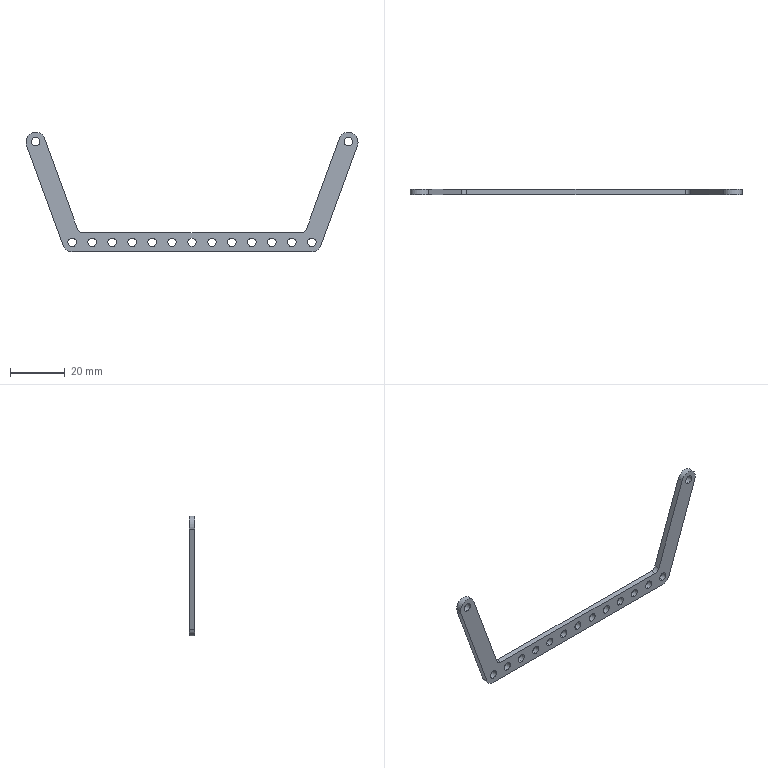Part | SolidWorks | features Extrusion 1, Fillet 1 | 1 solid | 44 faces | box 121 x 2 x 43.639 mm | volume 2162 mm3 | cylinder 36 | plane 8 | commonest cylinder face diameters 3.1 x30 7 x4 4 x2
STEP:
#1=CARTESIAN_POINT('',(57.,2.,-1.55));
#2=VERTEX_POINT('',#1);
#3=CARTESIAN_POINT('',(57.,2.,1.55));
#4=VERTEX_POINT('',#3);
#5=CARTESIAN_POINT('',(57.,2.,0.));
#6=DIRECTION('',(0.,1.,0.));
#7=DIRECTION('',(0.,0.,1.));
#8=AXIS2_PLACEMENT_3D('',#5,#6,#7);
#9=CIRCLE('',#8,1.55);
#10=EDGE_CURVE('',#2,#4,#9,.T.);
#11=ORIENTED_EDGE('',*,*,#10,.T.);
#12=CARTESIAN_POINT('',(57.,0.,1.55));
#13=VERTEX_POINT('',#12);
#14=CARTESIAN_POINT('',(57.,2.,1.55));
#15=DIRECTION('',(0.,-1.,0.));
#16=VECTOR('',#15,1000.);
#17=LINE('',#14,#16);
#18=EDGE_CURVE('',#4,#13,#17,.T.);
#19=ORIENTED_EDGE('',*,*,#18,.T.);
#20=CARTESIAN_POINT('',(57.,0.,-1.55));
#21=VERTEX_POINT('',#20);
#22=CARTESIAN_POINT('',(57.,0.,0.));
#23=DIRECTION('',(0.,1.,0.));
#24=DIRECTION('',(0.,0.,1.));
#25=AXIS2_PLACEMENT_3D('',#22,#23,#24);
#26=CIRCLE('',#25,1.55);
#27=EDGE_CURVE('',#21,#13,#26,.T.);
#28=ORIENTED_EDGE('',*,*,#27,.F.);
#29=CARTESIAN_POINT('',(57.,2.,-1.55));
#30=DIRECTION('',(0.,-1.,0.));
#31=VECTOR('',#30,1000.);
#32=LINE('',#29,#31);
#33=EDGE_CURVE('',#2,#21,#32,.T.);
#34=ORIENTED_EDGE('',*,*,#33,.F.);
#35=EDGE_LOOP('',(#11,#19,#28,#34));
#36=FACE_OUTER_BOUND('',#35,.T.);
#37=CARTESIAN_POINT('',(57.,2.,0.));
#38=DIRECTION('',(0.,-1.,0.));
#39=DIRECTION('',(0.,0.,-1.));
#40=AXIS2_PLACEMENT_3D('',#37,#38,#39);
#41=CYLINDRICAL_SURFACE('',#40,1.55);
#42=ADVANCED_FACE('',(#36),#41,.F.);
#43=CARTESIAN_POINT('',(-57.,2.,1.55));
#44=VERTEX_POINT('',#43);
#45=CARTESIAN_POINT('',(-57.,2.,-1.55));
#46=VERTEX_POINT('',#45);
#47=CARTESIAN_POINT('',(-57.,2.,0.));
#48=DIRECTION('',(0.,-1.,0.));
#49=DIRECTION('',(0.,0.,1.));
#50=AXIS2_PLACEMENT_3D('',#47,#48,#49);
#51=CIRCLE('',#50,1.55);
#52=EDGE_CURVE('',#44,#46,#51,.T.);
#53=ORIENTED_EDGE('',*,*,#52,.F.);
#54=CARTESIAN_POINT('',(-57.,0.,1.55));
#55=VERTEX_POINT('',#54);
#56=CARTESIAN_POINT('',(-57.,2.,1.55));
#57=DIRECTION('',(0.,-1.,0.));
#58=VECTOR('',#57,1000.);
#59=LINE('',#56,#58);
#60=EDGE_CURVE('',#44,#55,#59,.T.);
#61=ORIENTED_EDGE('',*,*,#60,.T.);
#62=CARTESIAN_POINT('',(-57.,0.,-1.55));
#63=VERTEX_POINT('',#62);
#64=CARTESIAN_POINT('',(-57.,0.,0.));
#65=DIRECTION('',(0.,-1.,0.));
#66=DIRECTION('',(0.,0.,1.));
#67=AXIS2_PLACEMENT_3D('',#64,#65,#66);
#68=CIRCLE('',#67,1.55);
#69=EDGE_CURVE('',#55,#63,#68,.T.);
#70=ORIENTED_EDGE('',*,*,#69,.T.);
#71=CARTESIAN_POINT('',(-57.,2.,-1.55));
#72=DIRECTION('',(0.,-1.,0.));
#73=VECTOR('',#72,1000.);
#74=LINE('',#71,#73);
#75=EDGE_CURVE('',#46,#63,#74,.T.);
#76=ORIENTED_EDGE('',*,*,#75,.F.);
#77=EDGE_LOOP('',(#53,#61,#70,#76));
#78=FACE_OUTER_BOUND('',#77,.T.);
#79=CARTESIAN_POINT('',(-57.,2.,0.));
#80=DIRECTION('',(0.,-1.,0.));
#81=DIRECTION('',(0.,0.,-1.));
#82=AXIS2_PLACEMENT_3D('',#79,#80,#81);
#83=CYLINDRICAL_SURFACE('',#82,1.55);
#84=ADVANCED_FACE('',(#78),#83,.F.);
#85=CARTESIAN_POINT('',(-43.665,2.,-35.089));
#86=VERTEX_POINT('',#85);
#87=CARTESIAN_POINT('',(-43.665,2.,-38.189));
#88=VERTEX_POINT('',#87);
#89=CARTESIAN_POINT('',(-43.665,2.,-36.639));
#90=DIRECTION('',(0.,-1.,0.));
#91=DIRECTION('',(0.,0.,1.));
#92=AXIS2_PLACEMENT_3D('',#89,#90,#91);
#93=CIRCLE('',#92,1.55);
#94=EDGE_CURVE('',#86,#88,#93,.T.);
#95=ORIENTED_EDGE('',*,*,#94,.F.);
#96=CARTESIAN_POINT('',(-43.665,0.,-35.089));
#97=VERTEX_POINT('',#96);
#98=CARTESIAN_POINT('',(-43.665,2.,-35.089));
#99=DIRECTION('',(0.,-1.,0.));
#100=VECTOR('',#99,1000.);
#101=LINE('',#98,#100);
#102=EDGE_CURVE('',#86,#97,#101,.T.);
#103=ORIENTED_EDGE('',*,*,#102,.T.);
#104=CARTESIAN_POINT('',(-43.665,0.,-38.189));
#105=VERTEX_POINT('',#104);
#106=CARTESIAN_POINT('',(-43.665,0.,-36.639));
#107=DIRECTION('',(0.,-1.,0.));
#108=DIRECTION('',(0.,0.,1.));
#109=AXIS2_PLACEMENT_3D('',#106,#107,#108);
#110=CIRCLE('',#109,1.55);
#111=EDGE_CURVE('',#97,#105,#110,.T.);
#112=ORIENTED_EDGE('',*,*,#111,.T.);
#113=CARTESIAN_POINT('',(-43.665,2.,-38.189));
#114=DIRECTION('',(0.,-1.,0.));
#115=VECTOR('',#114,1000.);
#116=LINE('',#113,#115);
#117=EDGE_CURVE('',#88,#105,#116,.T.);
#118=ORIENTED_EDGE('',*,*,#117,.F.);
#119=EDGE_LOOP('',(#95,#103,#112,#118));
#120=FACE_OUTER_BOUND('',#119,.T.);
#121=CARTESIAN_POINT('',(-43.665,2.,-36.639));
#122=DIRECTION('',(0.,-1.,0.));
#123=DIRECTION('',(0.,0.,-1.));
#124=AXIS2_PLACEMENT_3D('',#121,#122,#123);
#125=CYLINDRICAL_SURFACE('',#124,1.55);
#126=ADVANCED_FACE('',(#120),#125,.F.);
#127=CARTESIAN_POINT('',(36.388,2.,-38.189));
#128=VERTEX_POINT('',#127);
#129=CARTESIAN_POINT('',(36.388,2.,-35.089));
#130=VERTEX_POINT('',#129);
#131=CARTESIAN_POINT('',(36.388,2.,-36.639));
#132=DIRECTION('',(0.,1.,0.));
#133=DIRECTION('',(0.,0.,1.));
#134=AXIS2_PLACEMENT_3D('',#131,#132,#133);
#135=CIRCLE('',#134,1.55);
#136=EDGE_CURVE('',#128,#130,#135,.T.);
#137=ORIENTED_EDGE('',*,*,#136,.T.);
#138=CARTESIAN_POINT('',(36.388,0.,-35.089));
#139=VERTEX_POINT('',#138);
#140=CARTESIAN_POINT('',(36.388,2.,-35.089));
#141=DIRECTION('',(0.,-1.,0.));
#142=VECTOR('',#141,1000.);
#143=LINE('',#140,#142);
#144=EDGE_CURVE('',#130,#139,#143,.T.);
#145=ORIENTED_EDGE('',*,*,#144,.T.);
#146=CARTESIAN_POINT('',(36.388,0.,-38.189));
#147=VERTEX_POINT('',#146);
#148=CARTESIAN_POINT('',(36.388,0.,-36.639));
#149=DIRECTION('',(0.,1.,0.));
#150=DIRECTION('',(0.,0.,1.));
#151=AXIS2_PLACEMENT_3D('',#148,#149,#150);
#152=CIRCLE('',#151,1.55);
#153=EDGE_CURVE('',#147,#139,#152,.T.);
#154=ORIENTED_EDGE('',*,*,#153,.F.);
#155=CARTESIAN_POINT('',(36.388,2.,-38.189));
#156=DIRECTION('',(0.,-1.,0.));
#157=VECTOR('',#156,1000.);
#158=LINE('',#155,#157);
#159=EDGE_CURVE('',#128,#147,#158,.T.);
#160=ORIENTED_EDGE('',*,*,#159,.F.);
#161=EDGE_LOOP('',(#137,#145,#154,#160));
#162=FACE_OUTER_BOUND('',#161,.T.);
#163=CARTESIAN_POINT('',(36.388,2.,-36.639));
#164=DIRECTION('',(0.,-1.,0.));
#165=DIRECTION('',(0.,0.,-1.));
#166=AXIS2_PLACEMENT_3D('',#163,#164,#165);
#167=CYLINDRICAL_SURFACE('',#166,1.55);
#168=ADVANCED_FACE('',(#162),#167,.F.);
#169=CARTESIAN_POINT('',(29.111,2.,-38.189));
#170=VERTEX_POINT('',#169);
#171=CARTESIAN_POINT('',(29.111,2.,-35.089));
#172=VERTEX_POINT('',#171);
#173=CARTESIAN_POINT('',(29.111,2.,-36.639));
#174=DIRECTION('',(0.,1.,0.));
#175=DIRECTION('',(0.,0.,1.));
#176=AXIS2_PLACEMENT_3D('',#173,#174,#175);
#177=CIRCLE('',#176,1.55);
#178=EDGE_CURVE('',#170,#172,#177,.T.);
#179=ORIENTED_EDGE('',*,*,#178,.T.);
#180=CARTESIAN_POINT('',(29.111,0.,-35.089));
#181=VERTEX_POINT('',#180);
#182=CARTESIAN_POINT('',(29.111,2.,-35.089));
#183=DIRECTION('',(0.,-1.,0.));
#184=VECTOR('',#183,1000.);
#185=LINE('',#182,#184);
#186=EDGE_CURVE('',#172,#181,#185,.T.);
#187=ORIENTED_EDGE('',*,*,#186,.T.);
#188=CARTESIAN_POINT('',(29.111,0.,-38.189));
#189=VERTEX_POINT('',#188);
#190=CARTESIAN_POINT('',(29.111,0.,-36.639));
#191=DIRECTION('',(0.,1.,0.));
#192=DIRECTION('',(0.,0.,1.));
#193=AXIS2_PLACEMENT_3D('',#190,#191,#192);
#194=CIRCLE('',#193,1.55);
#195=EDGE_CURVE('',#189,#181,#194,.T.);
#196=ORIENTED_EDGE('',*,*,#195,.F.);
#197=CARTESIAN_POINT('',(29.111,2.,-38.189));
#198=DIRECTION('',(0.,-1.,0.));
#199=VECTOR('',#198,1000.);
#200=LINE('',#197,#199);
#201=EDGE_CURVE('',#170,#189,#200,.T.);
#202=ORIENTED_EDGE('',*,*,#201,.F.);
#203=EDGE_LOOP('',(#179,#187,#196,#202));
#204=FACE_OUTER_BOUND('',#203,.T.);
#205=CARTESIAN_POINT('',(29.111,2.,-36.639));
#206=DIRECTION('',(0.,-1.,0.));
#207=DIRECTION('',(0.,0.,-1.));
#208=AXIS2_PLACEMENT_3D('',#205,#206,#207);
#209=CYLINDRICAL_SURFACE('',#208,1.55);
#210=ADVANCED_FACE('',(#204),#209,.F.);
#211=CARTESIAN_POINT('',(21.834,2.,-38.189));
#212=VERTEX_POINT('',#211);
#213=CARTESIAN_POINT('',(21.834,2.,-35.089));
#214=VERTEX_POINT('',#213);
#215=CARTESIAN_POINT('',(21.834,2.,-36.639));
#216=DIRECTION('',(0.,1.,0.));
#217=DIRECTION('',(0.,0.,1.));
#218=AXIS2_PLACEMENT_3D('',#215,#216,#217);
#219=CIRCLE('',#218,1.55);
#220=EDGE_CURVE('',#212,#214,#219,.T.);
#221=ORIENTED_EDGE('',*,*,#220,.T.);
#222=CARTESIAN_POINT('',(21.834,0.,-35.089));
#223=VERTEX_POINT('',#222);
#224=CARTESIAN_POINT('',(21.834,2.,-35.089));
#225=DIRECTION('',(0.,-1.,0.));
#226=VECTOR('',#225,1000.);
#227=LINE('',#224,#226);
#228=EDGE_CURVE('',#214,#223,#227,.T.);
#229=ORIENTED_EDGE('',*,*,#228,.T.);
#230=CARTESIAN_POINT('',(21.834,0.,-38.189));
#231=VERTEX_POINT('',#230);
#232=CARTESIAN_POINT('',(21.834,0.,-36.639));
#233=DIRECTION('',(0.,1.,0.));
#234=DIRECTION('',(0.,0.,1.));
#235=AXIS2_PLACEMENT_3D('',#232,#233,#234);
#236=CIRCLE('',#235,1.55);
#237=EDGE_CURVE('',#231,#223,#236,.T.);
#238=ORIENTED_EDGE('',*,*,#237,.F.);
#239=CARTESIAN_POINT('',(21.834,2.,-38.189));
#240=DIRECTION('',(0.,-1.,0.));
#241=VECTOR('',#240,1000.);
#242=LINE('',#239,#241);
#243=EDGE_CURVE('',#212,#231,#242,.T.);
#244=ORIENTED_EDGE('',*,*,#243,.F.);
#245=EDGE_LOOP('',(#221,#229,#238,#244));
#246=FACE_OUTER_BOUND('',#245,.T.);
#247=CARTESIAN_POINT('',(21.834,2.,-36.639));
#248=DIRECTION('',(0.,-1.,0.));
#249=DIRECTION('',(0.,0.,-1.));
#250=AXIS2_PLACEMENT_3D('',#247,#248,#249);
#251=CYLINDRICAL_SURFACE('',#250,1.55);
#252=ADVANCED_FACE('',(#246),#251,.F.);
#253=CARTESIAN_POINT('',(14.557,2.,-38.189));
#254=VERTEX_POINT('',#253);
#255=CARTESIAN_POINT('',(14.557,2.,-35.089));
#256=VERTEX_POINT('',#255);
#257=CARTESIAN_POINT('',(14.557,2.,-36.639));
#258=DIRECTION('',(0.,1.,0.));
#259=DIRECTION('',(0.,0.,1.));
#260=AXIS2_PLACEMENT_3D('',#257,#258,#259);
#261=CIRCLE('',#260,1.55);
#262=EDGE_CURVE('',#254,#256,#261,.T.);
#263=ORIENTED_EDGE('',*,*,#262,.T.);
#264=CARTESIAN_POINT('',(14.557,0.,-35.089));
#265=VERTEX_POINT('',#264);
#266=CARTESIAN_POINT('',(14.557,2.,-35.089));
#267=DIRECTION('',(0.,-1.,0.));
#268=VECTOR('',#267,1000.);
#269=LINE('',#266,#268);
#270=EDGE_CURVE('',#256,#265,#269,.T.);
#271=ORIENTED_EDGE('',*,*,#270,.T.);
#272=CARTESIAN_POINT('',(14.557,0.,-38.189));
#273=VERTEX_POINT('',#272);
#274=CARTESIAN_POINT('',(14.557,0.,-36.639));
#275=DIRECTION('',(0.,1.,0.));
#276=DIRECTION('',(0.,0.,1.));
#277=AXIS2_PLACEMENT_3D('',#274,#275,#276);
#278=CIRCLE('',#277,1.55);
#279=EDGE_CURVE('',#273,#265,#278,.T.);
#280=ORIENTED_EDGE('',*,*,#279,.F.);
#281=CARTESIAN_POINT('',(14.557,2.,-38.189));
#282=DIRECTION('',(0.,-1.,0.));
#283=VECTOR('',#282,1000.);
#284=LINE('',#281,#283);
#285=EDGE_CURVE('',#254,#273,#284,.T.);
#286=ORIENTED_EDGE('',*,*,#285,.F.);
#287=EDGE_LOOP('',(#263,#271,#280,#286));
#288=FACE_OUTER_BOUND('',#287,.T.);
#289=CARTESIAN_POINT('',(14.557,2.,-36.639));
#290=DIRECTION('',(0.,-1.,0.));
#291=DIRECTION('',(0.,0.,-1.));
#292=AXIS2_PLACEMENT_3D('',#289,#290,#291);
#293=CYLINDRICAL_SURFACE('',#292,1.55);
#294=ADVANCED_FACE('',(#288),#293,.F.);
#295=CARTESIAN_POINT('',(7.28,2.,-38.189));
#296=VERTEX_POINT('',#295);
#297=CARTESIAN_POINT('',(7.28,2.,-35.089));
#298=VERTEX_POINT('',#297);
#299=CARTESIAN_POINT('',(7.28,2.,-36.639));
#300=DIRECTION('',(0.,1.,0.));
#301=DIRECTION('',(0.,0.,1.));
#302=AXIS2_PLACEMENT_3D('',#299,#300,#301);
#303=CIRCLE('',#302,1.55);
#304=EDGE_CURVE('',#296,#298,#303,.T.);
#305=ORIENTED_EDGE('',*,*,#304,.T.);
#306=CARTESIAN_POINT('',(7.28,0.,-35.089));
#307=VERTEX_POINT('',#306);
#308=CARTESIAN_POINT('',(7.28,2.,-35.089));
#309=DIRECTION('',(0.,-1.,0.));
#310=VECTOR('',#309,1000.);
#311=LINE('',#308,#310);
#312=EDGE_CURVE('',#298,#307,#311,.T.);
#313=ORIENTED_EDGE('',*,*,#312,.T.);
#314=CARTESIAN_POINT('',(7.28,0.,-38.189));
#315=VERTEX_POINT('',#314);
#316=CARTESIAN_POINT('',(7.28,0.,-36.639));
#317=DIRECTION('',(0.,1.,0.));
#318=DIRECTION('',(0.,0.,1.));
#319=AXIS2_PLACEMENT_3D('',#316,#317,#318);
#320=CIRCLE('',#319,1.55);
#321=EDGE_CURVE('',#315,#307,#320,.T.);
#322=ORIENTED_EDGE('',*,*,#321,.F.);
#323=CARTESIAN_POINT('',(7.28,2.,-38.189));
#324=DIRECTION('',(0.,-1.,0.));
#325=VECTOR('',#324,1000.);
#326=LINE('',#323,#325);
#327=EDGE_CURVE('',#296,#315,#326,.T.);
#328=ORIENTED_EDGE('',*,*,#327,.F.);
#329=EDGE_LOOP('',(#305,#313,#322,#328));
#330=FACE_OUTER_BOUND('',#329,.T.);
#331=CARTESIAN_POINT('',(7.28,2.,-36.639));
#332=DIRECTION('',(0.,-1.,0.));
#333=DIRECTION('',(0.,0.,-1.));
#334=AXIS2_PLACEMENT_3D('',#331,#332,#333);
#335=CYLINDRICAL_SURFACE('',#334,1.55);
#336=ADVANCED_FACE('',(#330),#335,.F.);
#337=CARTESIAN_POINT('',(-14.557,2.,-35.089));
#338=VERTEX_POINT('',#337);
#339=CARTESIAN_POINT('',(-14.557,2.,-38.189));
#340=VERTEX_POINT('',#339);
#341=CARTESIAN_POINT('',(-14.557,2.,-36.639));
#342=DIRECTION('',(0.,-1.,0.));
#343=DIRECTION('',(0.,0.,1.));
#344=AXIS2_PLACEMENT_3D('',#341,#342,#343);
#345=CIRCLE('',#344,1.55);
#346=EDGE_CURVE('',#338,#340,#345,.T.);
#347=ORIENTED_EDGE('',*,*,#346,.F.);
#348=CARTESIAN_POINT('',(-14.557,0.,-35.089));
#349=VERTEX_POINT('',#348);
#350=CARTESIAN_POINT('',(-14.557,2.,-35.089));
#351=DIRECTION('',(0.,-1.,0.));
#352=VECTOR('',#351,1000.);
#353=LINE('',#350,#352);
#354=EDGE_CURVE('',#338,#349,#353,.T.);
#355=ORIENTED_EDGE('',*,*,#354,.T.);
#356=CARTESIAN_POINT('',(-14.557,0.,-38.189));
#357=VERTEX_POINT('',#356);
#358=CARTESIAN_POINT('',(-14.557,0.,-36.639));
#359=DIRECTION('',(0.,-1.,0.));
#360=DIRECTION('',(0.,0.,1.));
#361=AXIS2_PLACEMENT_3D('',#358,#359,#360);
#362=CIRCLE('',#361,1.55);
#363=EDGE_CURVE('',#349,#357,#362,.T.);
#364=ORIENTED_EDGE('',*,*,#363,.T.);
#365=CARTESIAN_POINT('',(-14.557,2.,-38.189));
#366=DIRECTION('',(0.,-1.,0.));
#367=VECTOR('',#366,1000.);
#368=LINE('',#365,#367);
#369=EDGE_CURVE('',#340,#357,#368,.T.);
#370=ORIENTED_EDGE('',*,*,#369,.F.);
#371=EDGE_LOOP('',(#347,#355,#364,#370));
#372=FACE_OUTER_BOUND('',#371,.T.);
#373=CARTESIAN_POINT('',(-14.557,2.,-36.639));
#374=DIRECTION('',(0.,-1.,0.));
#375=DIRECTION('',(0.,0.,-1.));
#376=AXIS2_PLACEMENT_3D('',#373,#374,#375);
#377=CYLINDRICAL_SURFACE('',#376,1.55);
#378=ADVANCED_FACE('',(#372),#377,.F.);
#379=CARTESIAN_POINT('',(-29.111,2.,-35.089));
#380=VERTEX_POINT('',#379);
#381=CARTESIAN_POINT('',(-29.111,2.,-38.189));
#382=VERTEX_POINT('',#381);
#383=CARTESIAN_POINT('',(-29.111,2.,-36.639));
#384=DIRECTION('',(0.,-1.,0.));
#385=DIRECTION('',(0.,0.,1.));
#386=AXIS2_PLACEMENT_3D('',#383,#384,#385);
#387=CIRCLE('',#386,1.55);
#388=EDGE_CURVE('',#380,#382,#387,.T.);
#389=ORIENTED_EDGE('',*,*,#388,.F.);
#390=CARTESIAN_POINT('',(-29.111,0.,-35.089));
#391=VERTEX_POINT('',#390);
#392=CARTESIAN_POINT('',(-29.111,2.,-35.089));
#393=DIRECTION('',(0.,-1.,0.));
#394=VECTOR('',#393,1000.);
#395=LINE('',#392,#394);
#396=EDGE_CURVE('',#380,#391,#395,.T.);
#397=ORIENTED_EDGE('',*,*,#396,.T.);
#398=CARTESIAN_POINT('',(-29.111,0.,-38.189));
#399=VERTEX_POINT('',#398);
#400=CARTESIAN_POINT('',(-29.111,0.,-36.639));
#401=DIRECTION('',(0.,-1.,0.));
#402=DIRECTION('',(0.,0.,1.));
#403=AXIS2_PLACEMENT_3D('',#400,#401,#402);
#404=CIRCLE('',#403,1.55);
#405=EDGE_CURVE('',#391,#399,#404,.T.);
#406=ORIENTED_EDGE('',*,*,#405,.T.);
#407=CARTESIAN_POINT('',(-29.111,2.,-38.189));
#408=DIRECTION('',(0.,-1.,0.));
#409=VECTOR('',#408,1000.);
#410=LINE('',#407,#409);
#411=EDGE_CURVE('',#382,#399,#410,.T.);
#412=ORIENTED_EDGE('',*,*,#411,.F.);
#413=EDGE_LOOP('',(#389,#397,#406,#412));
#414=FACE_OUTER_BOUND('',#413,.T.);
#415=CARTESIAN_POINT('',(-29.111,2.,-36.639));
#416=DIRECTION('',(0.,-1.,0.));
#417=DIRECTION('',(0.,0.,-1.));
#418=AXIS2_PLACEMENT_3D('',#415,#416,#417);
#419=CYLINDRICAL_SURFACE('',#418,1.55);
#420=ADVANCED_FACE('',(#414),#419,.F.);
#421=CARTESIAN_POINT('',(0.,2.,-38.189));
#422=VERTEX_POINT('',#421);
#423=CARTESIAN_POINT('',(0.,2.,-35.089));
#424=VERTEX_POINT('',#423);
#425=CARTESIAN_POINT('',(0.,2.,-36.639));
#426=DIRECTION('',(0.,1.,0.));
#427=DIRECTION('',(0.,0.,1.));
#428=AXIS2_PLACEMENT_3D('',#425,#426,#427);
#429=CIRCLE('',#428,1.55);
#430=EDGE_CURVE('',#422,#424,#429,.T.);
#431=ORIENTED_EDGE('',*,*,#430,.T.);
#432=CARTESIAN_POINT('',(0.,0.,-35.089));
#433=VERTEX_POINT('',#432);
#434=CARTESIAN_POINT('',(0.,2.,-35.089));
#435=DIRECTION('',(0.,-1.,0.));
#436=VECTOR('',#435,1000.);
#437=LINE('',#434,#436);
#438=EDGE_CURVE('',#424,#433,#437,.T.);
#439=ORIENTED_EDGE('',*,*,#438,.T.);
#440=CARTESIAN_POINT('',(0.,0.,-38.189));
#441=VERTEX_POINT('',#440);
#442=CARTESIAN_POINT('',(0.,0.,-36.639));
#443=DIRECTION('',(0.,1.,0.));
#444=DIRECTION('',(0.,0.,1.));
#445=AXIS2_PLACEMENT_3D('',#442,#443,#444);
#446=CIRCLE('',#445,1.55);
#447=EDGE_CURVE('',#441,#433,#446,.T.);
#448=ORIENTED_EDGE('',*,*,#447,.F.);
#449=CARTESIAN_POINT('',(0.,2.,-38.189));
#450=DIRECTION('',(0.,-1.,0.));
#451=VECTOR('',#450,1000.);
#452=LINE('',#449,#451);
#453=EDGE_CURVE('',#422,#441,#452,.T.);
#454=ORIENTED_EDGE('',*,*,#453,.F.);
#455=EDGE_LOOP('',(#431,#439,#448,#454));
#456=FACE_OUTER_BOUND('',#455,.T.);
#457=CARTESIAN_POINT('',(0.,2.,-36.639));
#458=DIRECTION('',(0.,-1.,0.));
#459=DIRECTION('',(0.,0.,-1.));
#460=AXIS2_PLACEMENT_3D('',#457,#458,#459);
#461=CYLINDRICAL_SURFACE('',#460,1.55);
#462=ADVANCED_FACE('',(#456),#461,.F.);
#463=CARTESIAN_POINT('',(-36.388,2.,-35.089));
#464=VERTEX_POINT('',#463);
#465=CARTESIAN_POINT('',(-36.388,2.,-38.189));
#466=VERTEX_POINT('',#465);
#467=CARTESIAN_POINT('',(-36.388,2.,-36.639));
#468=DIRECTION('',(0.,-1.,0.));
#469=DIRECTION('',(0.,0.,1.));
#470=AXIS2_PLACEMENT_3D('',#467,#468,#469);
#471=CIRCLE('',#470,1.55);
#472=EDGE_CURVE('',#464,#466,#471,.T.);
#473=ORIENTED_EDGE('',*,*,#472,.F.);
#474=CARTESIAN_POINT('',(-36.388,0.,-35.089));
#475=VERTEX_POINT('',#474);
#476=CARTESIAN_POINT('',(-36.388,2.,-35.089));
#477=DIRECTION('',(0.,-1.,0.));
#478=VECTOR('',#477,1000.);
#479=LINE('',#476,#478);
#480=EDGE_CURVE('',#464,#475,#479,.T.);
#481=ORIENTED_EDGE('',*,*,#480,.T.);
#482=CARTESIAN_POINT('',(-36.388,0.,-38.189));
#483=VERTEX_POINT('',#482);
#484=CARTESIAN_POINT('',(-36.388,0.,-36.639));
#485=DIRECTION('',(0.,-1.,0.));
#486=DIRECTION('',(0.,0.,1.));
#487=AXIS2_PLACEMENT_3D('',#484,#485,#486);
#488=CIRCLE('',#487,1.55);
#489=EDGE_CURVE('',#475,#483,#488,.T.);
#490=ORIENTED_EDGE('',*,*,#489,.T.);
#491=CARTESIAN_POINT('',(-36.388,2.,-38.189));
#492=DIRECTION('',(0.,-1.,0.));
#493=VECTOR('',#492,1000.);
#494=LINE('',#491,#493);
#495=EDGE_CURVE('',#466,#483,#494,.T.);
#496=ORIENTED_EDGE('',*,*,#495,.F.);
#497=EDGE_LOOP('',(#473,#481,#490,#496));
#498=FACE_OUTER_BOUND('',#497,.T.);
#499=CARTESIAN_POINT('',(-36.388,2.,-36.639));
#500=DIRECTION('',(0.,-1.,0.));
#501=DIRECTION('',(0.,0.,-1.));
#502=AXIS2_PLACEMENT_3D('',#499,#500,#501);
#503=CYLINDRICAL_SURFACE('',#502,1.55);
#504=ADVANCED_FACE('',(#498),#503,.F.);
#505=CARTESIAN_POINT('',(-21.834,2.,-35.089));
#506=VERTEX_POINT('',#505);
#507=CARTESIAN_POINT('',(-21.834,2.,-38.189));
#508=VERTEX_POINT('',#507);
#509=CARTESIAN_POINT('',(-21.834,2.,-36.639));
#510=DIRECTION('',(0.,-1.,0.));
#511=DIRECTION('',(0.,0.,1.));
#512=AXIS2_PLACEMENT_3D('',#509,#510,#511);
#513=CIRCLE('',#512,1.55);
#514=EDGE_CURVE('',#506,#508,#513,.T.);
#515=ORIENTED_EDGE('',*,*,#514,.F.);
#516=CARTESIAN_POINT('',(-21.834,0.,-35.089));
#517=VERTEX_POINT('',#516);
#518=CARTESIAN_POINT('',(-21.834,2.,-35.089));
#519=DIRECTION('',(0.,-1.,0.));
#520=VECTOR('',#519,1000.);
#521=LINE('',#518,#520);
#522=EDGE_CURVE('',#506,#517,#521,.T.);
#523=ORIENTED_EDGE('',*,*,#522,.T.);
#524=CARTESIAN_POINT('',(-21.834,0.,-38.189));
#525=VERTEX_POINT('',#524);
#526=CARTESIAN_POINT('',(-21.834,0.,-36.639));
#527=DIRECTION('',(0.,-1.,0.));
#528=DIRECTION('',(0.,0.,1.));
#529=AXIS2_PLACEMENT_3D('',#526,#527,#528);
#530=CIRCLE('',#529,1.55);
#531=EDGE_CURVE('',#517,#525,#530,.T.);
#532=ORIENTED_EDGE('',*,*,#531,.T.);
#533=CARTESIAN_POINT('',(-21.834,2.,-38.189));
#534=DIRECTION('',(0.,-1.,0.));
#535=VECTOR('',#534,1000.);
#536=LINE('',#533,#535);
#537=EDGE_CURVE('',#508,#525,#536,.T.);
#538=ORIENTED_EDGE('',*,*,#537,.F.);
#539=EDGE_LOOP('',(#515,#523,#532,#538));
#540=FACE_OUTER_BOUND('',#539,.T.);
#541=CARTESIAN_POINT('',(-21.834,2.,-36.639));
#542=DIRECTION('',(0.,-1.,0.));
#543=DIRECTION('',(0.,0.,-1.));
#544=AXIS2_PLACEMENT_3D('',#541,#542,#543);
#545=CYLINDRICAL_SURFACE('',#544,1.55);
#546=ADVANCED_FACE('',(#540),#545,.F.);
#547=CARTESIAN_POINT('',(-7.28,2.,-35.089));
#548=VERTEX_POINT('',#547);
#549=CARTESIAN_POINT('',(-7.28,2.,-38.189));
#550=VERTEX_POINT('',#549);
#551=CARTESIAN_POINT('',(-7.28,2.,-36.639));
#552=DIRECTION('',(0.,-1.,0.));
#553=DIRECTION('',(0.,0.,1.));
#554=AXIS2_PLACEMENT_3D('',#551,#552,#553);
#555=CIRCLE('',#554,1.55);
#556=EDGE_CURVE('',#548,#550,#555,.T.);
#557=ORIENTED_EDGE('',*,*,#556,.F.);
#558=CARTESIAN_POINT('',(-7.28,0.,-35.089));
#559=VERTEX_POINT('',#558);
#560=CARTESIAN_POINT('',(-7.28,2.,-35.089));
#561=DIRECTION('',(0.,-1.,0.));
#562=VECTOR('',#561,1000.);
#563=LINE('',#560,#562);
#564=EDGE_CURVE('',#548,#559,#563,.T.);
#565=ORIENTED_EDGE('',*,*,#564,.T.);
#566=CARTESIAN_POINT('',(-7.28,0.,-38.189));
#567=VERTEX_POINT('',#566);
#568=CARTESIAN_POINT('',(-7.28,0.,-36.639));
#569=DIRECTION('',(0.,-1.,0.));
#570=DIRECTION('',(0.,0.,1.));
#571=AXIS2_PLACEMENT_3D('',#568,#569,#570);
#572=CIRCLE('',#571,1.55);
#573=EDGE_CURVE('',#559,#567,#572,.T.);
#574=ORIENTED_EDGE('',*,*,#573,.T.);
#575=CARTESIAN_POINT('',(-7.28,2.,-38.189));
#576=DIRECTION('',(0.,-1.,0.));
#577=VECTOR('',#576,1000.);
#578=LINE('',#575,#577);
#579=EDGE_CURVE('',#550,#567,#578,.T.);
#580=ORIENTED_EDGE('',*,*,#579,.F.);
#581=EDGE_LOOP('',(#557,#565,#574,#580));
#582=FACE_OUTER_BOUND('',#581,.T.);
#583=CARTESIAN_POINT('',(-7.28,2.,-36.639));
#584=DIRECTION('',(0.,-1.,0.));
#585=DIRECTION('',(0.,0.,-1.));
#586=AXIS2_PLACEMENT_3D('',#583,#584,#585);
#587=CYLINDRICAL_SURFACE('',#586,1.55);
#588=ADVANCED_FACE('',(#582),#587,.F.);
#589=CARTESIAN_POINT('',(43.665,2.,-38.189));
#590=VERTEX_POINT('',#589);
#591=CARTESIAN_POINT('',(43.665,2.,-35.089));
#592=VERTEX_POINT('',#591);
#593=CARTESIAN_POINT('',(43.665,2.,-36.639));
#594=DIRECTION('',(0.,1.,0.));
#595=DIRECTION('',(0.,0.,1.));
#596=AXIS2_PLACEMENT_3D('',#593,#594,#595);
#597=CIRCLE('',#596,1.55);
#598=EDGE_CURVE('',#590,#592,#597,.T.);
#599=ORIENTED_EDGE('',*,*,#598,.T.);
#600=CARTESIAN_POINT('',(43.665,0.,-35.089));
#601=VERTEX_POINT('',#600);
#602=CARTESIAN_POINT('',(43.665,2.,-35.089));
#603=DIRECTION('',(0.,-1.,0.));
#604=VECTOR('',#603,1000.);
#605=LINE('',#602,#604);
#606=EDGE_CURVE('',#592,#601,#605,.T.);
#607=ORIENTED_EDGE('',*,*,#606,.T.);
#608=CARTESIAN_POINT('',(43.665,0.,-38.189));
#609=VERTEX_POINT('',#608);
#610=CARTESIAN_POINT('',(43.665,0.,-36.639));
#611=DIRECTION('',(0.,1.,0.));
#612=DIRECTION('',(0.,0.,1.));
#613=AXIS2_PLACEMENT_3D('',#610,#611,#612);
#614=CIRCLE('',#613,1.55);
#615=EDGE_CURVE('',#609,#601,#614,.T.);
#616=ORIENTED_EDGE('',*,*,#615,.F.);
#617=CARTESIAN_POINT('',(43.665,2.,-38.189));
#618=DIRECTION('',(0.,-1.,0.));
#619=VECTOR('',#618,1000.);
#620=LINE('',#617,#619);
#621=EDGE_CURVE('',#590,#609,#620,.T.);
#622=ORIENTED_EDGE('',*,*,#621,.F.);
#623=EDGE_LOOP('',(#599,#607,#616,#622));
#624=FACE_OUTER_BOUND('',#623,.T.);
#625=CARTESIAN_POINT('',(43.665,2.,-36.639));
#626=DIRECTION('',(0.,-1.,0.));
#627=DIRECTION('',(0.,0.,-1.));
#628=AXIS2_PLACEMENT_3D('',#625,#626,#627);
#629=CYLINDRICAL_SURFACE('',#628,1.55);
#630=ADVANCED_FACE('',(#624),#629,.F.);
#631=CARTESIAN_POINT('',(-39.813,0.,-33.139));
#632=VERTEX_POINT('',#631);
#633=CARTESIAN_POINT('',(39.813,0.,-33.139));
#634=VERTEX_POINT('',#633);
#635=CARTESIAN_POINT('',(0.,0.,-33.139));
#636=DIRECTION('',(1.,0.,0.));
#637=VECTOR('',#636,1000.);
#638=LINE('',#635,#637);
#639=EDGE_CURVE('',#632,#634,#638,.T.);
#640=ORIENTED_EDGE('',*,*,#639,.T.);
#641=CARTESIAN_POINT('',(39.813,2.,-33.139));
#642=VERTEX_POINT('',#641);
#643=CARTESIAN_POINT('',(39.813,2.,-33.139));
#644=DIRECTION('',(0.,1.,0.));
#645=VECTOR('',#644,1000.);
#646=LINE('',#643,#645);
#647=EDGE_CURVE('',#634,#642,#646,.T.);
#648=ORIENTED_EDGE('',*,*,#647,.T.);
#649=CARTESIAN_POINT('',(-39.813,2.,-33.139));
#650=VERTEX_POINT('',#649);
#651=CARTESIAN_POINT('',(0.,2.,-33.139));
#652=DIRECTION('',(1.,0.,0.));
#653=VECTOR('',#652,1000.);
#654=LINE('',#651,#653);
#655=EDGE_CURVE('',#650,#642,#654,.T.);
#656=ORIENTED_EDGE('',*,*,#655,.F.);
#657=CARTESIAN_POINT('',(-39.813,0.,-33.139));
#658=DIRECTION('',(0.,-1.,0.));
#659=VECTOR('',#658,1000.);
#660=LINE('',#657,#659);
#661=EDGE_CURVE('',#650,#632,#660,.T.);
#662=ORIENTED_EDGE('',*,*,#661,.T.);
#663=EDGE_LOOP('',(#640,#648,#656,#662));
#664=FACE_OUTER_BOUND('',#663,.T.);
#665=CARTESIAN_POINT('',(0.,2.,-33.139));
#666=DIRECTION('',(0.,0.,-1.));
#667=DIRECTION('',(-1.,0.,0.));
#668=AXIS2_PLACEMENT_3D('',#665,#666,#667);
#669=PLANE('',#668);
#670=ADVANCED_FACE('',(#664),#669,.F.);
#671=CARTESIAN_POINT('',(41.693,2.,-31.823));
#672=VERTEX_POINT('',#671);
#673=CARTESIAN_POINT('',(53.711,2.,1.197));
#674=VERTEX_POINT('',#673);
#675=CARTESIAN_POINT('',(47.043,2.,-17.122));
#676=DIRECTION('',(0.342,0.,0.9397));
#677=VECTOR('',#676,1000.);
#678=LINE('',#675,#677);
#679=EDGE_CURVE('',#672,#674,#678,.T.);
#680=ORIENTED_EDGE('',*,*,#679,.F.);
#681=CARTESIAN_POINT('',(41.693,0.,-31.823));
#682=VERTEX_POINT('',#681);
#683=CARTESIAN_POINT('',(41.693,0.,-31.823));
#684=DIRECTION('',(0.,-1.,0.));
#685=VECTOR('',#684,1000.);
#686=LINE('',#683,#685);
#687=EDGE_CURVE('',#672,#682,#686,.T.);
#688=ORIENTED_EDGE('',*,*,#687,.T.);
#689=CARTESIAN_POINT('',(53.711,0.,1.197));
#690=VERTEX_POINT('',#689);
#691=CARTESIAN_POINT('',(47.043,0.,-17.122));
#692=DIRECTION('',(0.342,0.,0.9397));
#693=VECTOR('',#692,1000.);
#694=LINE('',#691,#693);
#695=EDGE_CURVE('',#682,#690,#694,.T.);
#696=ORIENTED_EDGE('',*,*,#695,.T.);
#697=CARTESIAN_POINT('',(53.711,2.,1.197));
#698=DIRECTION('',(0.,-1.,0.));
#699=VECTOR('',#698,1000.);
#700=LINE('',#697,#699);
#701=EDGE_CURVE('',#674,#690,#700,.T.);
#702=ORIENTED_EDGE('',*,*,#701,.F.);
#703=EDGE_LOOP('',(#680,#688,#696,#702));
#704=FACE_OUTER_BOUND('',#703,.T.);
#705=CARTESIAN_POINT('',(47.043,2.,-17.122));
#706=DIRECTION('',(0.9397,0.,-0.342));
#707=DIRECTION('',(-0.342,0.,-0.9397));
#708=AXIS2_PLACEMENT_3D('',#705,#706,#707);
#709=PLANE('',#708);
#710=ADVANCED_FACE('',(#704),#709,.F.);
#711=CARTESIAN_POINT('',(60.289,0.,-1.197));
#712=VERTEX_POINT('',#711);
#713=CARTESIAN_POINT('',(57.,0.,0.));
#714=DIRECTION('',(0.,1.,0.));
#715=DIRECTION('',(0.,0.,1.));
#716=AXIS2_PLACEMENT_3D('',#713,#714,#715);
#717=CIRCLE('',#716,3.5);
#718=EDGE_CURVE('',#690,#712,#717,.T.);
#719=ORIENTED_EDGE('',*,*,#718,.T.);
#720=CARTESIAN_POINT('',(60.289,2.,-1.197));
#721=VERTEX_POINT('',#720);
#722=CARTESIAN_POINT('',(60.289,2.,-1.197));
#723=DIRECTION('',(0.,-1.,0.));
#724=VECTOR('',#723,1000.);
#725=LINE('',#722,#724);
#726=EDGE_CURVE('',#721,#712,#725,.T.);
#727=ORIENTED_EDGE('',*,*,#726,.F.);
#728=CARTESIAN_POINT('',(57.,2.,0.));
#729=DIRECTION('',(0.,1.,0.));
#730=DIRECTION('',(0.,0.,1.));
#731=AXIS2_PLACEMENT_3D('',#728,#729,#730);
#732=CIRCLE('',#731,3.5);
#733=EDGE_CURVE('',#674,#721,#732,.T.);
#734=ORIENTED_EDGE('',*,*,#733,.F.);
#735=ORIENTED_EDGE('',*,*,#701,.T.);
#736=EDGE_LOOP('',(#719,#727,#734,#735));
#737=FACE_OUTER_BOUND('',#736,.T.);
#738=CARTESIAN_POINT('',(57.,2.,0.));
#739=DIRECTION('',(0.,-1.,0.));
#740=DIRECTION('',(0.,0.,-1.));
#741=AXIS2_PLACEMENT_3D('',#738,#739,#740);
#742=CYLINDRICAL_SURFACE('',#741,3.5);
#743=ADVANCED_FACE('',(#737),#742,.T.);
#744=CARTESIAN_POINT('',(46.953,0.,-37.836));
#745=VERTEX_POINT('',#744);
#746=CARTESIAN_POINT('',(53.621,0.,-19.517));
#747=DIRECTION('',(0.342,0.,0.9397));
#748=VECTOR('',#747,1000.);
#749=LINE('',#746,#748);
#750=EDGE_CURVE('',#745,#712,#749,.T.);
#751=ORIENTED_EDGE('',*,*,#750,.F.);
#752=CARTESIAN_POINT('',(46.953,2.,-37.836));
#753=VERTEX_POINT('',#752);
#754=CARTESIAN_POINT('',(46.953,2.,-37.836));
#755=DIRECTION('',(0.,-1.,0.));
#756=VECTOR('',#755,1000.);
#757=LINE('',#754,#756);
#758=EDGE_CURVE('',#753,#745,#757,.T.);
#759=ORIENTED_EDGE('',*,*,#758,.F.);
#760=CARTESIAN_POINT('',(53.621,2.,-19.517));
#761=DIRECTION('',(0.342,0.,0.9397));
#762=VECTOR('',#761,1000.);
#763=LINE('',#760,#762);
#764=EDGE_CURVE('',#753,#721,#763,.T.);
#765=ORIENTED_EDGE('',*,*,#764,.T.);
#766=ORIENTED_EDGE('',*,*,#726,.T.);
#767=EDGE_LOOP('',(#751,#759,#765,#766));
#768=FACE_OUTER_BOUND('',#767,.T.);
#769=CARTESIAN_POINT('',(53.621,2.,-19.517));
#770=DIRECTION('',(0.9397,0.,-0.342));
#771=DIRECTION('',(-0.342,0.,-0.9397));
#772=AXIS2_PLACEMENT_3D('',#769,#770,#771);
#773=PLANE('',#772);
#774=ADVANCED_FACE('',(#768),#773,.T.);
#775=CARTESIAN_POINT('',(43.665,0.,-40.139));
#776=VERTEX_POINT('',#775);
#777=CARTESIAN_POINT('',(43.665,0.,-36.639));
#778=DIRECTION('',(0.,1.,0.));
#779=DIRECTION('',(0.,0.,1.));
#780=AXIS2_PLACEMENT_3D('',#777,#778,#779);
#781=CIRCLE('',#780,3.5);
#782=EDGE_CURVE('',#745,#776,#781,.T.);
#783=ORIENTED_EDGE('',*,*,#782,.T.);
#784=CARTESIAN_POINT('',(43.665,2.,-40.139));
#785=VERTEX_POINT('',#784);
#786=CARTESIAN_POINT('',(43.665,2.,-40.139));
#787=DIRECTION('',(0.,-1.,0.));
#788=VECTOR('',#787,1000.);
#789=LINE('',#786,#788);
#790=EDGE_CURVE('',#785,#776,#789,.T.);
#791=ORIENTED_EDGE('',*,*,#790,.F.);
#792=CARTESIAN_POINT('',(43.665,2.,-36.639));
#793=DIRECTION('',(0.,1.,0.));
#794=DIRECTION('',(0.,0.,1.));
#795=AXIS2_PLACEMENT_3D('',#792,#793,#794);
#796=CIRCLE('',#795,3.5);
#797=EDGE_CURVE('',#753,#785,#796,.T.);
#798=ORIENTED_EDGE('',*,*,#797,.F.);
#799=ORIENTED_EDGE('',*,*,#758,.T.);
#800=EDGE_LOOP('',(#783,#791,#798,#799));
#801=FACE_OUTER_BOUND('',#800,.T.);
#802=CARTESIAN_POINT('',(43.665,2.,-36.639));
#803=DIRECTION('',(0.,-1.,0.));
#804=DIRECTION('',(0.,0.,-1.));
#805=AXIS2_PLACEMENT_3D('',#802,#803,#804);
#806=CYLINDRICAL_SURFACE('',#805,3.5);
#807=ADVANCED_FACE('',(#801),#806,.T.);
#808=CARTESIAN_POINT('',(-43.665,0.,-40.139));
#809=VERTEX_POINT('',#808);
#810=CARTESIAN_POINT('',(0.,0.,-40.139));
#811=DIRECTION('',(1.,0.,0.));
#812=VECTOR('',#811,1000.);
#813=LINE('',#810,#812);
#814=EDGE_CURVE('',#809,#776,#813,.T.);
#815=ORIENTED_EDGE('',*,*,#814,.F.);
#816=CARTESIAN_POINT('',(-43.665,2.,-40.139));
#817=VERTEX_POINT('',#816);
#818=CARTESIAN_POINT('',(-43.665,2.,-40.139));
#819=DIRECTION('',(0.,-1.,0.));
#820=VECTOR('',#819,1000.);
#821=LINE('',#818,#820);
#822=EDGE_CURVE('',#817,#809,#821,.T.);
#823=ORIENTED_EDGE('',*,*,#822,.F.);
#824=CARTESIAN_POINT('',(0.,2.,-40.139));
#825=DIRECTION('',(1.,0.,0.));
#826=VECTOR('',#825,1000.);
#827=LINE('',#824,#826);
#828=EDGE_CURVE('',#817,#785,#827,.T.);
#829=ORIENTED_EDGE('',*,*,#828,.T.);
#830=ORIENTED_EDGE('',*,*,#790,.T.);
#831=EDGE_LOOP('',(#815,#823,#829,#830));
#832=FACE_OUTER_BOUND('',#831,.T.);
#833=CARTESIAN_POINT('',(0.,2.,-40.139));
#834=DIRECTION('',(0.,0.,-1.));
#835=DIRECTION('',(-1.,0.,0.));
#836=AXIS2_PLACEMENT_3D('',#833,#834,#835);
#837=PLANE('',#836);
#838=ADVANCED_FACE('',(#832),#837,.T.);
#839=CARTESIAN_POINT('',(-46.953,0.,-37.836));
#840=VERTEX_POINT('',#839);
#841=CARTESIAN_POINT('',(-43.665,0.,-36.639));
#842=DIRECTION('',(0.,1.,0.));
#843=DIRECTION('',(0.,0.,1.));
#844=AXIS2_PLACEMENT_3D('',#841,#842,#843);
#845=CIRCLE('',#844,3.5);
#846=EDGE_CURVE('',#809,#840,#845,.T.);
#847=ORIENTED_EDGE('',*,*,#846,.T.);
#848=CARTESIAN_POINT('',(-46.953,2.,-37.836));
#849=VERTEX_POINT('',#848);
#850=CARTESIAN_POINT('',(-46.953,2.,-37.836));
#851=DIRECTION('',(0.,-1.,0.));
#852=VECTOR('',#851,1000.);
#853=LINE('',#850,#852);
#854=EDGE_CURVE('',#849,#840,#853,.T.);
#855=ORIENTED_EDGE('',*,*,#854,.F.);
#856=CARTESIAN_POINT('',(-43.665,2.,-36.639));
#857=DIRECTION('',(0.,1.,0.));
#858=DIRECTION('',(0.,0.,1.));
#859=AXIS2_PLACEMENT_3D('',#856,#857,#858);
#860=CIRCLE('',#859,3.5);
#861=EDGE_CURVE('',#817,#849,#860,.T.);
#862=ORIENTED_EDGE('',*,*,#861,.F.);
#863=ORIENTED_EDGE('',*,*,#822,.T.);
#864=EDGE_LOOP('',(#847,#855,#862,#863));
#865=FACE_OUTER_BOUND('',#864,.T.);
#866=CARTESIAN_POINT('',(-43.665,2.,-36.639));
#867=DIRECTION('',(0.,-1.,0.));
#868=DIRECTION('',(0.,0.,-1.));
#869=AXIS2_PLACEMENT_3D('',#866,#867,#868);
#870=CYLINDRICAL_SURFACE('',#869,3.5);
#871=ADVANCED_FACE('',(#865),#870,.T.);
#872=CARTESIAN_POINT('',(-60.289,0.,-1.197));
#873=VERTEX_POINT('',#872);
#874=CARTESIAN_POINT('',(-53.621,0.,-19.517));
#875=DIRECTION('',(0.342,0.,-0.9397));
#876=VECTOR('',#875,1000.);
#877=LINE('',#874,#876);
#878=EDGE_CURVE('',#873,#840,#877,.T.);
#879=ORIENTED_EDGE('',*,*,#878,.F.);
#880=CARTESIAN_POINT('',(-60.289,2.,-1.197));
#881=VERTEX_POINT('',#880);
#882=CARTESIAN_POINT('',(-60.289,2.,-1.197));
#883=DIRECTION('',(0.,-1.,0.));
#884=VECTOR('',#883,1000.);
#885=LINE('',#882,#884);
#886=EDGE_CURVE('',#881,#873,#885,.T.);
#887=ORIENTED_EDGE('',*,*,#886,.F.);
#888=CARTESIAN_POINT('',(-53.621,2.,-19.517));
#889=DIRECTION('',(0.342,0.,-0.9397));
#890=VECTOR('',#889,1000.);
#891=LINE('',#888,#890);
#892=EDGE_CURVE('',#881,#849,#891,.T.);
#893=ORIENTED_EDGE('',*,*,#892,.T.);
#894=ORIENTED_EDGE('',*,*,#854,.T.);
#895=EDGE_LOOP('',(#879,#887,#893,#894));
#896=FACE_OUTER_BOUND('',#895,.T.);
#897=CARTESIAN_POINT('',(-53.621,2.,-19.517));
#898=DIRECTION('',(-0.9397,0.,-0.342));
#899=DIRECTION('',(-0.342,0.,0.9397));
#900=AXIS2_PLACEMENT_3D('',#897,#898,#899);
#901=PLANE('',#900);
#902=ADVANCED_FACE('',(#896),#901,.T.);
#903=CARTESIAN_POINT('',(-53.711,0.,1.197));
#904=VERTEX_POINT('',#903);
#905=CARTESIAN_POINT('',(-57.,0.,0.));
#906=DIRECTION('',(0.,1.,0.));
#907=DIRECTION('',(0.,0.,1.));
#908=AXIS2_PLACEMENT_3D('',#905,#906,#907);
#909=CIRCLE('',#908,3.5);
#910=EDGE_CURVE('',#873,#904,#909,.T.);
#911=ORIENTED_EDGE('',*,*,#910,.T.);
#912=CARTESIAN_POINT('',(-53.711,2.,1.197));
#913=VERTEX_POINT('',#912);
#914=CARTESIAN_POINT('',(-53.711,2.,1.197));
#915=DIRECTION('',(0.,-1.,0.));
#916=VECTOR('',#915,1000.);
#917=LINE('',#914,#916);
#918=EDGE_CURVE('',#913,#904,#917,.T.);
#919=ORIENTED_EDGE('',*,*,#918,.F.);
#920=CARTESIAN_POINT('',(-57.,2.,0.));
#921=DIRECTION('',(0.,1.,0.));
#922=DIRECTION('',(0.,0.,1.));
#923=AXIS2_PLACEMENT_3D('',#920,#921,#922);
#924=CIRCLE('',#923,3.5);
#925=EDGE_CURVE('',#881,#913,#924,.T.);
#926=ORIENTED_EDGE('',*,*,#925,.F.);
#927=ORIENTED_EDGE('',*,*,#886,.T.);
#928=EDGE_LOOP('',(#911,#919,#926,#927));
#929=FACE_OUTER_BOUND('',#928,.T.);
#930=CARTESIAN_POINT('',(-57.,2.,0.));
#931=DIRECTION('',(0.,-1.,0.));
#932=DIRECTION('',(0.,0.,-1.));
#933=AXIS2_PLACEMENT_3D('',#930,#931,#932);
#934=CYLINDRICAL_SURFACE('',#933,3.5);
#935=ADVANCED_FACE('',(#929),#934,.T.);
#936=ORIENTED_EDGE('',*,*,#606,.F.);
#937=CARTESIAN_POINT('',(43.665,2.,-36.639));
#938=DIRECTION('',(0.,1.,0.));
#939=DIRECTION('',(0.,0.,1.));
#940=AXIS2_PLACEMENT_3D('',#937,#938,#939);
#941=CIRCLE('',#940,1.55);
#942=EDGE_CURVE('',#592,#590,#941,.T.);
#943=ORIENTED_EDGE('',*,*,#942,.T.);
#944=ORIENTED_EDGE('',*,*,#621,.T.);
#945=CARTESIAN_POINT('',(43.665,0.,-36.639));
#946=DIRECTION('',(0.,1.,0.));
#947=DIRECTION('',(0.,0.,1.));
#948=AXIS2_PLACEMENT_3D('',#945,#946,#947);
#949=CIRCLE('',#948,1.55);
#950=EDGE_CURVE('',#601,#609,#949,.T.);
#951=ORIENTED_EDGE('',*,*,#950,.F.);
#952=EDGE_LOOP('',(#936,#943,#944,#951));
#953=FACE_OUTER_BOUND('',#952,.T.);
#954=CARTESIAN_POINT('',(43.665,2.,-36.639));
#955=DIRECTION('',(0.,-1.,0.));
#956=DIRECTION('',(0.,0.,-1.));
#957=AXIS2_PLACEMENT_3D('',#954,#955,#956);
#958=CYLINDRICAL_SURFACE('',#957,1.55);
#959=ADVANCED_FACE('',(#953),#958,.F.);
#960=ORIENTED_EDGE('',*,*,#564,.F.);
#961=CARTESIAN_POINT('',(-7.28,2.,-36.639));
#962=DIRECTION('',(0.,-1.,0.));
#963=DIRECTION('',(0.,0.,1.));
#964=AXIS2_PLACEMENT_3D('',#961,#962,#963);
#965=CIRCLE('',#964,1.55);
#966=EDGE_CURVE('',#550,#548,#965,.T.);
#967=ORIENTED_EDGE('',*,*,#966,.F.);
#968=ORIENTED_EDGE('',*,*,#579,.T.);
#969=CARTESIAN_POINT('',(-7.28,0.,-36.639));
#970=DIRECTION('',(0.,-1.,0.));
#971=DIRECTION('',(0.,0.,1.));
#972=AXIS2_PLACEMENT_3D('',#969,#970,#971);
#973=CIRCLE('',#972,1.55);
#974=EDGE_CURVE('',#567,#559,#973,.T.);
#975=ORIENTED_EDGE('',*,*,#974,.T.);
#976=EDGE_LOOP('',(#960,#967,#968,#975));
#977=FACE_OUTER_BOUND('',#976,.T.);
#978=CARTESIAN_POINT('',(-7.28,2.,-36.639));
#979=DIRECTION('',(0.,-1.,0.));
#980=DIRECTION('',(0.,0.,-1.));
#981=AXIS2_PLACEMENT_3D('',#978,#979,#980);
#982=CYLINDRICAL_SURFACE('',#981,1.55);
#983=ADVANCED_FACE('',(#977),#982,.F.);
#984=ORIENTED_EDGE('',*,*,#522,.F.);
#985=CARTESIAN_POINT('',(-21.834,2.,-36.639));
#986=DIRECTION('',(0.,-1.,0.));
#987=DIRECTION('',(0.,0.,1.));
#988=AXIS2_PLACEMENT_3D('',#985,#986,#987);
#989=CIRCLE('',#988,1.55);
#990=EDGE_CURVE('',#508,#506,#989,.T.);
#991=ORIENTED_EDGE('',*,*,#990,.F.);
#992=ORIENTED_EDGE('',*,*,#537,.T.);
#993=CARTESIAN_POINT('',(-21.834,0.,-36.639));
#994=DIRECTION('',(0.,-1.,0.));
#995=DIRECTION('',(0.,0.,1.));
#996=AXIS2_PLACEMENT_3D('',#993,#994,#995);
#997=CIRCLE('',#996,1.55);
#998=EDGE_CURVE('',#525,#517,#997,.T.);
#999=ORIENTED_EDGE('',*,*,#998,.T.);
#1000=EDGE_LOOP('',(#984,#991,#992,#999));
#1001=FACE_OUTER_BOUND('',#1000,.T.);
#1002=CARTESIAN_POINT('',(-21.834,2.,-36.639));
#1003=DIRECTION('',(0.,-1.,0.));
#1004=DIRECTION('',(0.,0.,-1.));
#1005=AXIS2_PLACEMENT_3D('',#1002,#1003,#1004);
#1006=CYLINDRICAL_SURFACE('',#1005,1.55);
#1007=ADVANCED_FACE('',(#1001),#1006,.F.);
#1008=ORIENTED_EDGE('',*,*,#480,.F.);
#1009=CARTESIAN_POINT('',(-36.388,2.,-36.639));
#1010=DIRECTION('',(0.,-1.,0.));
#1011=DIRECTION('',(0.,0.,1.));
#1012=AXIS2_PLACEMENT_3D('',#1009,#1010,#1011);
#1013=CIRCLE('',#1012,1.55);
#1014=EDGE_CURVE('',#466,#464,#1013,.T.);
#1015=ORIENTED_EDGE('',*,*,#1014,.F.);
#1016=ORIENTED_EDGE('',*,*,#495,.T.);
#1017=CARTESIAN_POINT('',(-36.388,0.,-36.639));
#1018=DIRECTION('',(0.,-1.,0.));
#1019=DIRECTION('',(0.,0.,1.));
#1020=AXIS2_PLACEMENT_3D('',#1017,#1018,#1019);
#1021=CIRCLE('',#1020,1.55);
#1022=EDGE_CURVE('',#483,#475,#1021,.T.);
#1023=ORIENTED_EDGE('',*,*,#1022,.T.);
#1024=EDGE_LOOP('',(#1008,#1015,#1016,#1023));
#1025=FACE_OUTER_BOUND('',#1024,.T.);
#1026=CARTESIAN_POINT('',(-36.388,2.,-36.639));
#1027=DIRECTION('',(0.,-1.,0.));
#1028=DIRECTION('',(0.,0.,-1.));
#1029=AXIS2_PLACEMENT_3D('',#1026,#1027,#1028);
#1030=CYLINDRICAL_SURFACE('',#1029,1.55);
#1031=ADVANCED_FACE('',(#1025),#1030,.F.);
#1032=ORIENTED_EDGE('',*,*,#438,.F.);
#1033=CARTESIAN_POINT('',(0.,2.,-36.639));
#1034=DIRECTION('',(0.,1.,0.));
#1035=DIRECTION('',(0.,0.,1.));
#1036=AXIS2_PLACEMENT_3D('',#1033,#1034,#1035);
#1037=CIRCLE('',#1036,1.55);
#1038=EDGE_CURVE('',#424,#422,#1037,.T.);
#1039=ORIENTED_EDGE('',*,*,#1038,.T.);
#1040=ORIENTED_EDGE('',*,*,#453,.T.);
#1041=CARTESIAN_POINT('',(0.,0.,-36.639));
#1042=DIRECTION('',(0.,1.,0.));
#1043=DIRECTION('',(0.,0.,1.));
#1044=AXIS2_PLACEMENT_3D('',#1041,#1042,#1043);
#1045=CIRCLE('',#1044,1.55);
#1046=EDGE_CURVE('',#433,#441,#1045,.T.);
#1047=ORIENTED_EDGE('',*,*,#1046,.F.);
#1048=EDGE_LOOP('',(#1032,#1039,#1040,#1047));
#1049=FACE_OUTER_BOUND('',#1048,.T.);
#1050=CARTESIAN_POINT('',(0.,2.,-36.639));
#1051=DIRECTION('',(0.,-1.,0.));
#1052=DIRECTION('',(0.,0.,-1.));
#1053=AXIS2_PLACEMENT_3D('',#1050,#1051,#1052);
#1054=CYLINDRICAL_SURFACE('',#1053,1.55);
#1055=ADVANCED_FACE('',(#1049),#1054,.F.);
#1056=ORIENTED_EDGE('',*,*,#396,.F.);
#1057=CARTESIAN_POINT('',(-29.111,2.,-36.639));
#1058=DIRECTION('',(0.,-1.,0.));
#1059=DIRECTION('',(0.,0.,1.));
#1060=AXIS2_PLACEMENT_3D('',#1057,#1058,#1059);
#1061=CIRCLE('',#1060,1.55);
#1062=EDGE_CURVE('',#382,#380,#1061,.T.);
#1063=ORIENTED_EDGE('',*,*,#1062,.F.);
#1064=ORIENTED_EDGE('',*,*,#411,.T.);
#1065=CARTESIAN_POINT('',(-29.111,0.,-36.639));
#1066=DIRECTION('',(0.,-1.,0.));
#1067=DIRECTION('',(0.,0.,1.));
#1068=AXIS2_PLACEMENT_3D('',#1065,#1066,#1067);
#1069=CIRCLE('',#1068,1.55);
#1070=EDGE_CURVE('',#399,#391,#1069,.T.);
#1071=ORIENTED_EDGE('',*,*,#1070,.T.);
#1072=EDGE_LOOP('',(#1056,#1063,#1064,#1071));
#1073=FACE_OUTER_BOUND('',#1072,.T.);
#1074=CARTESIAN_POINT('',(-29.111,2.,-36.639));
#1075=DIRECTION('',(0.,-1.,0.));
#1076=DIRECTION('',(0.,0.,-1.));
#1077=AXIS2_PLACEMENT_3D('',#1074,#1075,#1076);
#1078=CYLINDRICAL_SURFACE('',#1077,1.55);
#1079=ADVANCED_FACE('',(#1073),#1078,.F.);
#1080=ORIENTED_EDGE('',*,*,#354,.F.);
#1081=CARTESIAN_POINT('',(-14.557,2.,-36.639));
#1082=DIRECTION('',(0.,-1.,0.));
#1083=DIRECTION('',(0.,0.,1.));
#1084=AXIS2_PLACEMENT_3D('',#1081,#1082,#1083);
#1085=CIRCLE('',#1084,1.55);
#1086=EDGE_CURVE('',#340,#338,#1085,.T.);
#1087=ORIENTED_EDGE('',*,*,#1086,.F.);
#1088=ORIENTED_EDGE('',*,*,#369,.T.);
#1089=CARTESIAN_POINT('',(-14.557,0.,-36.639));
#1090=DIRECTION('',(0.,-1.,0.));
#1091=DIRECTION('',(0.,0.,1.));
#1092=AXIS2_PLACEMENT_3D('',#1089,#1090,#1091);
#1093=CIRCLE('',#1092,1.55);
#1094=EDGE_CURVE('',#357,#349,#1093,.T.);
#1095=ORIENTED_EDGE('',*,*,#1094,.T.);
#1096=EDGE_LOOP('',(#1080,#1087,#1088,#1095));
#1097=FACE_OUTER_BOUND('',#1096,.T.);
#1098=CARTESIAN_POINT('',(-14.557,2.,-36.639));
#1099=DIRECTION('',(0.,-1.,0.));
#1100=DIRECTION('',(0.,0.,-1.));
#1101=AXIS2_PLACEMENT_3D('',#1098,#1099,#1100);
#1102=CYLINDRICAL_SURFACE('',#1101,1.55);
#1103=ADVANCED_FACE('',(#1097),#1102,.F.);
#1104=ORIENTED_EDGE('',*,*,#312,.F.);
#1105=CARTESIAN_POINT('',(7.28,2.,-36.639));
#1106=DIRECTION('',(0.,1.,0.));
#1107=DIRECTION('',(0.,0.,1.));
#1108=AXIS2_PLACEMENT_3D('',#1105,#1106,#1107);
#1109=CIRCLE('',#1108,1.55);
#1110=EDGE_CURVE('',#298,#296,#1109,.T.);
#1111=ORIENTED_EDGE('',*,*,#1110,.T.);
#1112=ORIENTED_EDGE('',*,*,#327,.T.);
#1113=CARTESIAN_POINT('',(7.28,0.,-36.639));
#1114=DIRECTION('',(0.,1.,0.));
#1115=DIRECTION('',(0.,0.,1.));
#1116=AXIS2_PLACEMENT_3D('',#1113,#1114,#1115);
#1117=CIRCLE('',#1116,1.55);
#1118=EDGE_CURVE('',#307,#315,#1117,.T.);
#1119=ORIENTED_EDGE('',*,*,#1118,.F.);
#1120=EDGE_LOOP('',(#1104,#1111,#1112,#1119));
#1121=FACE_OUTER_BOUND('',#1120,.T.);
#1122=CARTESIAN_POINT('',(7.28,2.,-36.639));
#1123=DIRECTION('',(0.,-1.,0.));
#1124=DIRECTION('',(0.,0.,-1.));
#1125=AXIS2_PLACEMENT_3D('',#1122,#1123,#1124);
#1126=CYLINDRICAL_SURFACE('',#1125,1.55);
#1127=ADVANCED_FACE('',(#1121),#1126,.F.);
#1128=ORIENTED_EDGE('',*,*,#270,.F.);
#1129=CARTESIAN_POINT('',(14.557,2.,-36.639));
#1130=DIRECTION('',(0.,1.,0.));
#1131=DIRECTION('',(0.,0.,1.));
#1132=AXIS2_PLACEMENT_3D('',#1129,#1130,#1131);
#1133=CIRCLE('',#1132,1.55);
#1134=EDGE_CURVE('',#256,#254,#1133,.T.);
#1135=ORIENTED_EDGE('',*,*,#1134,.T.);
#1136=ORIENTED_EDGE('',*,*,#285,.T.);
#1137=CARTESIAN_POINT('',(14.557,0.,-36.639));
#1138=DIRECTION('',(0.,1.,0.));
#1139=DIRECTION('',(0.,0.,1.));
#1140=AXIS2_PLACEMENT_3D('',#1137,#1138,#1139);
#1141=CIRCLE('',#1140,1.55);
#1142=EDGE_CURVE('',#265,#273,#1141,.T.);
#1143=ORIENTED_EDGE('',*,*,#1142,.F.);
#1144=EDGE_LOOP('',(#1128,#1135,#1136,#1143));
#1145=FACE_OUTER_BOUND('',#1144,.T.);
#1146=CARTESIAN_POINT('',(14.557,2.,-36.639));
#1147=DIRECTION('',(0.,-1.,0.));
#1148=DIRECTION('',(0.,0.,-1.));
#1149=AXIS2_PLACEMENT_3D('',#1146,#1147,#1148);
#1150=CYLINDRICAL_SURFACE('',#1149,1.55);
#1151=ADVANCED_FACE('',(#1145),#1150,.F.);
#1152=ORIENTED_EDGE('',*,*,#228,.F.);
#1153=CARTESIAN_POINT('',(21.834,2.,-36.639));
#1154=DIRECTION('',(0.,1.,0.));
#1155=DIRECTION('',(0.,0.,1.));
#1156=AXIS2_PLACEMENT_3D('',#1153,#1154,#1155);
#1157=CIRCLE('',#1156,1.55);
#1158=EDGE_CURVE('',#214,#212,#1157,.T.);
#1159=ORIENTED_EDGE('',*,*,#1158,.T.);
#1160=ORIENTED_EDGE('',*,*,#243,.T.);
#1161=CARTESIAN_POINT('',(21.834,0.,-36.639));
#1162=DIRECTION('',(0.,1.,0.));
#1163=DIRECTION('',(0.,0.,1.));
#1164=AXIS2_PLACEMENT_3D('',#1161,#1162,#1163);
#1165=CIRCLE('',#1164,1.55);
#1166=EDGE_CURVE('',#223,#231,#1165,.T.);
#1167=ORIENTED_EDGE('',*,*,#1166,.F.);
#1168=EDGE_LOOP('',(#1152,#1159,#1160,#1167));
#1169=FACE_OUTER_BOUND('',#1168,.T.);
#1170=CARTESIAN_POINT('',(21.834,2.,-36.639));
#1171=DIRECTION('',(0.,-1.,0.));
#1172=DIRECTION('',(0.,0.,-1.));
#1173=AXIS2_PLACEMENT_3D('',#1170,#1171,#1172);
#1174=CYLINDRICAL_SURFACE('',#1173,1.55);
#1175=ADVANCED_FACE('',(#1169),#1174,.F.);
#1176=ORIENTED_EDGE('',*,*,#186,.F.);
#1177=CARTESIAN_POINT('',(29.111,2.,-36.639));
#1178=DIRECTION('',(0.,1.,0.));
#1179=DIRECTION('',(0.,0.,1.));
#1180=AXIS2_PLACEMENT_3D('',#1177,#1178,#1179);
#1181=CIRCLE('',#1180,1.55);
#1182=EDGE_CURVE('',#172,#170,#1181,.T.);
#1183=ORIENTED_EDGE('',*,*,#1182,.T.);
#1184=ORIENTED_EDGE('',*,*,#201,.T.);
#1185=CARTESIAN_POINT('',(29.111,0.,-36.639));
#1186=DIRECTION('',(0.,1.,0.));
#1187=DIRECTION('',(0.,0.,1.));
#1188=AXIS2_PLACEMENT_3D('',#1185,#1186,#1187);
#1189=CIRCLE('',#1188,1.55);
#1190=EDGE_CURVE('',#181,#189,#1189,.T.);
#1191=ORIENTED_EDGE('',*,*,#1190,.F.);
#1192=EDGE_LOOP('',(#1176,#1183,#1184,#1191));
#1193=FACE_OUTER_BOUND('',#1192,.T.);
#1194=CARTESIAN_POINT('',(29.111,2.,-36.639));
#1195=DIRECTION('',(0.,-1.,0.));
#1196=DIRECTION('',(0.,0.,-1.));
#1197=AXIS2_PLACEMENT_3D('',#1194,#1195,#1196);
#1198=CYLINDRICAL_SURFACE('',#1197,1.55);
#1199=ADVANCED_FACE('',(#1193),#1198,.F.);
#1200=ORIENTED_EDGE('',*,*,#144,.F.);
#1201=CARTESIAN_POINT('',(36.388,2.,-36.639));
#1202=DIRECTION('',(0.,1.,0.));
#1203=DIRECTION('',(0.,0.,1.));
#1204=AXIS2_PLACEMENT_3D('',#1201,#1202,#1203);
#1205=CIRCLE('',#1204,1.55);
#1206=EDGE_CURVE('',#130,#128,#1205,.T.);
#1207=ORIENTED_EDGE('',*,*,#1206,.T.);
#1208=ORIENTED_EDGE('',*,*,#159,.T.);
#1209=CARTESIAN_POINT('',(36.388,0.,-36.639));
#1210=DIRECTION('',(0.,1.,0.));
#1211=DIRECTION('',(0.,0.,1.));
#1212=AXIS2_PLACEMENT_3D('',#1209,#1210,#1211);
#1213=CIRCLE('',#1212,1.55);
#1214=EDGE_CURVE('',#139,#147,#1213,.T.);
#1215=ORIENTED_EDGE('',*,*,#1214,.F.);
#1216=EDGE_LOOP('',(#1200,#1207,#1208,#1215));
#1217=FACE_OUTER_BOUND('',#1216,.T.);
#1218=CARTESIAN_POINT('',(36.388,2.,-36.639));
#1219=DIRECTION('',(0.,-1.,0.));
#1220=DIRECTION('',(0.,0.,-1.));
#1221=AXIS2_PLACEMENT_3D('',#1218,#1219,#1220);
#1222=CYLINDRICAL_SURFACE('',#1221,1.55);
#1223=ADVANCED_FACE('',(#1217),#1222,.F.);
#1224=ORIENTED_EDGE('',*,*,#102,.F.);
#1225=CARTESIAN_POINT('',(-43.665,2.,-36.639));
#1226=DIRECTION('',(0.,-1.,0.));
#1227=DIRECTION('',(0.,0.,1.));
#1228=AXIS2_PLACEMENT_3D('',#1225,#1226,#1227);
#1229=CIRCLE('',#1228,1.55);
#1230=EDGE_CURVE('',#88,#86,#1229,.T.);
#1231=ORIENTED_EDGE('',*,*,#1230,.F.);
#1232=ORIENTED_EDGE('',*,*,#117,.T.);
#1233=CARTESIAN_POINT('',(-43.665,0.,-36.639));
#1234=DIRECTION('',(0.,-1.,0.));
#1235=DIRECTION('',(0.,0.,1.));
#1236=AXIS2_PLACEMENT_3D('',#1233,#1234,#1235);
#1237=CIRCLE('',#1236,1.55);
#1238=EDGE_CURVE('',#105,#97,#1237,.T.);
#1239=ORIENTED_EDGE('',*,*,#1238,.T.);
#1240=EDGE_LOOP('',(#1224,#1231,#1232,#1239));
#1241=FACE_OUTER_BOUND('',#1240,.T.);
#1242=CARTESIAN_POINT('',(-43.665,2.,-36.639));
#1243=DIRECTION('',(0.,-1.,0.));
#1244=DIRECTION('',(0.,0.,-1.));
#1245=AXIS2_PLACEMENT_3D('',#1242,#1243,#1244);
#1246=CYLINDRICAL_SURFACE('',#1245,1.55);
#1247=ADVANCED_FACE('',(#1241),#1246,.F.);
#1248=ORIENTED_EDGE('',*,*,#60,.F.);
#1249=CARTESIAN_POINT('',(-57.,2.,0.));
#1250=DIRECTION('',(0.,-1.,0.));
#1251=DIRECTION('',(0.,0.,1.));
#1252=AXIS2_PLACEMENT_3D('',#1249,#1250,#1251);
#1253=CIRCLE('',#1252,1.55);
#1254=EDGE_CURVE('',#46,#44,#1253,.T.);
#1255=ORIENTED_EDGE('',*,*,#1254,.F.);
#1256=ORIENTED_EDGE('',*,*,#75,.T.);
#1257=CARTESIAN_POINT('',(-57.,0.,0.));
#1258=DIRECTION('',(0.,-1.,0.));
#1259=DIRECTION('',(0.,0.,1.));
#1260=AXIS2_PLACEMENT_3D('',#1257,#1258,#1259);
#1261=CIRCLE('',#1260,1.55);
#1262=EDGE_CURVE('',#63,#55,#1261,.T.);
#1263=ORIENTED_EDGE('',*,*,#1262,.T.);
#1264=EDGE_LOOP('',(#1248,#1255,#1256,#1263));
#1265=FACE_OUTER_BOUND('',#1264,.T.);
#1266=CARTESIAN_POINT('',(-57.,2.,0.));
#1267=DIRECTION('',(0.,-1.,0.));
#1268=DIRECTION('',(0.,0.,-1.));
#1269=AXIS2_PLACEMENT_3D('',#1266,#1267,#1268);
#1270=CYLINDRICAL_SURFACE('',#1269,1.55);
#1271=ADVANCED_FACE('',(#1265),#1270,.F.);
#1272=CARTESIAN_POINT('',(-41.693,0.,-31.823));
#1273=VERTEX_POINT('',#1272);
#1274=CARTESIAN_POINT('',(-47.043,0.,-17.122));
#1275=DIRECTION('',(0.342,0.,-0.9397));
#1276=VECTOR('',#1275,1000.);
#1277=LINE('',#1274,#1276);
#1278=EDGE_CURVE('',#904,#1273,#1277,.T.);
#1279=ORIENTED_EDGE('',*,*,#1278,.T.);
#1280=CARTESIAN_POINT('',(-41.693,2.,-31.823));
#1281=VERTEX_POINT('',#1280);
#1282=CARTESIAN_POINT('',(-41.693,2.,-31.823));
#1283=DIRECTION('',(0.,1.,0.));
#1284=VECTOR('',#1283,1000.);
#1285=LINE('',#1282,#1284);
#1286=EDGE_CURVE('',#1273,#1281,#1285,.T.);
#1287=ORIENTED_EDGE('',*,*,#1286,.T.);
#1288=CARTESIAN_POINT('',(-47.043,2.,-17.122));
#1289=DIRECTION('',(0.342,0.,-0.9397));
#1290=VECTOR('',#1289,1000.);
#1291=LINE('',#1288,#1290);
#1292=EDGE_CURVE('',#913,#1281,#1291,.T.);
#1293=ORIENTED_EDGE('',*,*,#1292,.F.);
#1294=ORIENTED_EDGE('',*,*,#918,.T.);
#1295=EDGE_LOOP('',(#1279,#1287,#1293,#1294));
#1296=FACE_OUTER_BOUND('',#1295,.T.);
#1297=CARTESIAN_POINT('',(-47.043,2.,-17.122));
#1298=DIRECTION('',(-0.9397,0.,-0.342));
#1299=DIRECTION('',(-0.342,0.,0.9397));
#1300=AXIS2_PLACEMENT_3D('',#1297,#1298,#1299);
#1301=PLANE('',#1300);
#1302=ADVANCED_FACE('',(#1296),#1301,.F.);
#1303=ORIENTED_EDGE('',*,*,#18,.F.);
#1304=CARTESIAN_POINT('',(57.,2.,0.));
#1305=DIRECTION('',(0.,1.,0.));
#1306=DIRECTION('',(0.,0.,1.));
#1307=AXIS2_PLACEMENT_3D('',#1304,#1305,#1306);
#1308=CIRCLE('',#1307,1.55);
#1309=EDGE_CURVE('',#4,#2,#1308,.T.);
#1310=ORIENTED_EDGE('',*,*,#1309,.T.);
#1311=ORIENTED_EDGE('',*,*,#33,.T.);
#1312=CARTESIAN_POINT('',(57.,0.,0.));
#1313=DIRECTION('',(0.,1.,0.));
#1314=DIRECTION('',(0.,0.,1.));
#1315=AXIS2_PLACEMENT_3D('',#1312,#1313,#1314);
#1316=CIRCLE('',#1315,1.55);
#1317=EDGE_CURVE('',#13,#21,#1316,.T.);
#1318=ORIENTED_EDGE('',*,*,#1317,.F.);
#1319=EDGE_LOOP('',(#1303,#1310,#1311,#1318));
#1320=FACE_OUTER_BOUND('',#1319,.T.);
#1321=CARTESIAN_POINT('',(57.,2.,0.));
#1322=DIRECTION('',(0.,-1.,0.));
#1323=DIRECTION('',(0.,0.,-1.));
#1324=AXIS2_PLACEMENT_3D('',#1321,#1322,#1323);
#1325=CYLINDRICAL_SURFACE('',#1324,1.55);
#1326=ADVANCED_FACE('',(#1320),#1325,.F.);
#1327=ORIENTED_EDGE('',*,*,#1292,.T.);
#1328=CARTESIAN_POINT('',(-39.813,2.,-31.139));
#1329=DIRECTION('',(0.,-1.,0.));
#1330=DIRECTION('',(0.,0.,1.));
#1331=AXIS2_PLACEMENT_3D('',#1328,#1329,#1330);
#1332=CIRCLE('',#1331,2.);
#1333=EDGE_CURVE('',#1281,#650,#1332,.T.);
#1334=ORIENTED_EDGE('',*,*,#1333,.T.);
#1335=ORIENTED_EDGE('',*,*,#655,.T.);
#1336=CARTESIAN_POINT('',(39.813,2.,-31.139));
#1337=DIRECTION('',(0.,-1.,0.));
#1338=DIRECTION('',(0.,0.,1.));
#1339=AXIS2_PLACEMENT_3D('',#1336,#1337,#1338);
#1340=CIRCLE('',#1339,2.);
#1341=EDGE_CURVE('',#642,#672,#1340,.T.);
#1342=ORIENTED_EDGE('',*,*,#1341,.T.);
#1343=ORIENTED_EDGE('',*,*,#679,.T.);
#1344=ORIENTED_EDGE('',*,*,#733,.T.);
#1345=ORIENTED_EDGE('',*,*,#764,.F.);
#1346=ORIENTED_EDGE('',*,*,#797,.T.);
#1347=ORIENTED_EDGE('',*,*,#828,.F.);
#1348=ORIENTED_EDGE('',*,*,#861,.T.);
#1349=ORIENTED_EDGE('',*,*,#892,.F.);
#1350=ORIENTED_EDGE('',*,*,#925,.T.);
#1351=EDGE_LOOP('',(#1327,#1334,#1335,#1342,#1343,#1344,#1345,#1346,#1347,#1348,#1349,#1350));
#1352=FACE_OUTER_BOUND('',#1351,.T.);
#1353=ORIENTED_EDGE('',*,*,#1254,.T.);
#1354=ORIENTED_EDGE('',*,*,#52,.T.);
#1355=EDGE_LOOP('',(#1353,#1354));
#1356=FACE_BOUND('',#1355,.T.);
#1357=ORIENTED_EDGE('',*,*,#1230,.T.);
#1358=ORIENTED_EDGE('',*,*,#94,.T.);
#1359=EDGE_LOOP('',(#1357,#1358));
#1360=FACE_BOUND('',#1359,.T.);
#1361=ORIENTED_EDGE('',*,*,#136,.F.);
#1362=ORIENTED_EDGE('',*,*,#1206,.F.);
#1363=EDGE_LOOP('',(#1361,#1362));
#1364=FACE_BOUND('',#1363,.T.);
#1365=ORIENTED_EDGE('',*,*,#178,.F.);
#1366=ORIENTED_EDGE('',*,*,#1182,.F.);
#1367=EDGE_LOOP('',(#1365,#1366));
#1368=FACE_BOUND('',#1367,.T.);
#1369=ORIENTED_EDGE('',*,*,#220,.F.);
#1370=ORIENTED_EDGE('',*,*,#1158,.F.);
#1371=EDGE_LOOP('',(#1369,#1370));
#1372=FACE_BOUND('',#1371,.T.);
#1373=ORIENTED_EDGE('',*,*,#262,.F.);
#1374=ORIENTED_EDGE('',*,*,#1134,.F.);
#1375=EDGE_LOOP('',(#1373,#1374));
#1376=FACE_BOUND('',#1375,.T.);
#1377=ORIENTED_EDGE('',*,*,#304,.F.);
#1378=ORIENTED_EDGE('',*,*,#1110,.F.);
#1379=EDGE_LOOP('',(#1377,#1378));
#1380=FACE_BOUND('',#1379,.T.);
#1381=ORIENTED_EDGE('',*,*,#1086,.T.);
#1382=ORIENTED_EDGE('',*,*,#346,.T.);
#1383=EDGE_LOOP('',(#1381,#1382));
#1384=FACE_BOUND('',#1383,.T.);
#1385=ORIENTED_EDGE('',*,*,#1062,.T.);
#1386=ORIENTED_EDGE('',*,*,#388,.T.);
#1387=EDGE_LOOP('',(#1385,#1386));
#1388=FACE_BOUND('',#1387,.T.);
#1389=ORIENTED_EDGE('',*,*,#430,.F.);
#1390=ORIENTED_EDGE('',*,*,#1038,.F.);
#1391=EDGE_LOOP('',(#1389,#1390));
#1392=FACE_BOUND('',#1391,.T.);
#1393=ORIENTED_EDGE('',*,*,#1014,.T.);
#1394=ORIENTED_EDGE('',*,*,#472,.T.);
#1395=EDGE_LOOP('',(#1393,#1394));
#1396=FACE_BOUND('',#1395,.T.);
#1397=ORIENTED_EDGE('',*,*,#990,.T.);
#1398=ORIENTED_EDGE('',*,*,#514,.T.);
#1399=EDGE_LOOP('',(#1397,#1398));
#1400=FACE_BOUND('',#1399,.T.);
#1401=ORIENTED_EDGE('',*,*,#966,.T.);
#1402=ORIENTED_EDGE('',*,*,#556,.T.);
#1403=EDGE_LOOP('',(#1401,#1402));
#1404=FACE_BOUND('',#1403,.T.);
#1405=ORIENTED_EDGE('',*,*,#598,.F.);
#1406=ORIENTED_EDGE('',*,*,#942,.F.);
#1407=EDGE_LOOP('',(#1405,#1406));
#1408=FACE_BOUND('',#1407,.T.);
#1409=ORIENTED_EDGE('',*,*,#10,.F.);
#1410=ORIENTED_EDGE('',*,*,#1309,.F.);
#1411=EDGE_LOOP('',(#1409,#1410));
#1412=FACE_BOUND('',#1411,.T.);
#1413=CARTESIAN_POINT('',(0.,2.,0.));
#1414=DIRECTION('',(0.,1.,0.));
#1415=DIRECTION('',(0.,0.,1.));
#1416=AXIS2_PLACEMENT_3D('',#1413,#1414,#1415);
#1417=PLANE('',#1416);
#1418=ADVANCED_FACE('',(#1352,#1356,#1360,#1364,#1368,#1372,#1376,#1380,#1384,#1388,#1392,#1396,#1400,#1404,#1408,#1412),#1417,.T.);
#1419=ORIENTED_EDGE('',*,*,#639,.F.);
#1420=CARTESIAN_POINT('',(-39.813,0.,-31.139));
#1421=DIRECTION('',(0.,1.,0.));
#1422=DIRECTION('',(0.,0.,1.));
#1423=AXIS2_PLACEMENT_3D('',#1420,#1421,#1422);
#1424=CIRCLE('',#1423,2.);
#1425=EDGE_CURVE('',#632,#1273,#1424,.T.);
#1426=ORIENTED_EDGE('',*,*,#1425,.T.);
#1427=ORIENTED_EDGE('',*,*,#1278,.F.);
#1428=ORIENTED_EDGE('',*,*,#910,.F.);
#1429=ORIENTED_EDGE('',*,*,#878,.T.);
#1430=ORIENTED_EDGE('',*,*,#846,.F.);
#1431=ORIENTED_EDGE('',*,*,#814,.T.);
#1432=ORIENTED_EDGE('',*,*,#782,.F.);
#1433=ORIENTED_EDGE('',*,*,#750,.T.);
#1434=ORIENTED_EDGE('',*,*,#718,.F.);
#1435=ORIENTED_EDGE('',*,*,#695,.F.);
#1436=CARTESIAN_POINT('',(39.813,0.,-31.139));
#1437=DIRECTION('',(0.,1.,0.));
#1438=DIRECTION('',(0.,0.,1.));
#1439=AXIS2_PLACEMENT_3D('',#1436,#1437,#1438);
#1440=CIRCLE('',#1439,2.);
#1441=EDGE_CURVE('',#682,#634,#1440,.T.);
#1442=ORIENTED_EDGE('',*,*,#1441,.T.);
#1443=EDGE_LOOP('',(#1419,#1426,#1427,#1428,#1429,#1430,#1431,#1432,#1433,#1434,#1435,#1442));
#1444=FACE_OUTER_BOUND('',#1443,.T.);
#1445=ORIENTED_EDGE('',*,*,#1262,.F.);
#1446=ORIENTED_EDGE('',*,*,#69,.F.);
#1447=EDGE_LOOP('',(#1445,#1446));
#1448=FACE_BOUND('',#1447,.T.);
#1449=ORIENTED_EDGE('',*,*,#1238,.F.);
#1450=ORIENTED_EDGE('',*,*,#111,.F.);
#1451=EDGE_LOOP('',(#1449,#1450));
#1452=FACE_BOUND('',#1451,.T.);
#1453=ORIENTED_EDGE('',*,*,#153,.T.);
#1454=ORIENTED_EDGE('',*,*,#1214,.T.);
#1455=EDGE_LOOP('',(#1453,#1454));
#1456=FACE_BOUND('',#1455,.T.);
#1457=ORIENTED_EDGE('',*,*,#195,.T.);
#1458=ORIENTED_EDGE('',*,*,#1190,.T.);
#1459=EDGE_LOOP('',(#1457,#1458));
#1460=FACE_BOUND('',#1459,.T.);
#1461=ORIENTED_EDGE('',*,*,#237,.T.);
#1462=ORIENTED_EDGE('',*,*,#1166,.T.);
#1463=EDGE_LOOP('',(#1461,#1462));
#1464=FACE_BOUND('',#1463,.T.);
#1465=ORIENTED_EDGE('',*,*,#279,.T.);
#1466=ORIENTED_EDGE('',*,*,#1142,.T.);
#1467=EDGE_LOOP('',(#1465,#1466));
#1468=FACE_BOUND('',#1467,.T.);
#1469=ORIENTED_EDGE('',*,*,#321,.T.);
#1470=ORIENTED_EDGE('',*,*,#1118,.T.);
#1471=EDGE_LOOP('',(#1469,#1470));
#1472=FACE_BOUND('',#1471,.T.);
#1473=ORIENTED_EDGE('',*,*,#1094,.F.);
#1474=ORIENTED_EDGE('',*,*,#363,.F.);
#1475=EDGE_LOOP('',(#1473,#1474));
#1476=FACE_BOUND('',#1475,.T.);
#1477=ORIENTED_EDGE('',*,*,#1070,.F.);
#1478=ORIENTED_EDGE('',*,*,#405,.F.);
#1479=EDGE_LOOP('',(#1477,#1478));
#1480=FACE_BOUND('',#1479,.T.);
#1481=ORIENTED_EDGE('',*,*,#447,.T.);
#1482=ORIENTED_EDGE('',*,*,#1046,.T.);
#1483=EDGE_LOOP('',(#1481,#1482));
#1484=FACE_BOUND('',#1483,.T.);
#1485=ORIENTED_EDGE('',*,*,#1022,.F.);
#1486=ORIENTED_EDGE('',*,*,#489,.F.);
#1487=EDGE_LOOP('',(#1485,#1486));
#1488=FACE_BOUND('',#1487,.T.);
#1489=ORIENTED_EDGE('',*,*,#998,.F.);
#1490=ORIENTED_EDGE('',*,*,#531,.F.);
#1491=EDGE_LOOP('',(#1489,#1490));
#1492=FACE_BOUND('',#1491,.T.);
#1493=ORIENTED_EDGE('',*,*,#974,.F.);
#1494=ORIENTED_EDGE('',*,*,#573,.F.);
#1495=EDGE_LOOP('',(#1493,#1494));
#1496=FACE_BOUND('',#1495,.T.);
#1497=ORIENTED_EDGE('',*,*,#615,.T.);
#1498=ORIENTED_EDGE('',*,*,#950,.T.);
#1499=EDGE_LOOP('',(#1497,#1498));
#1500=FACE_BOUND('',#1499,.T.);
#1501=ORIENTED_EDGE('',*,*,#27,.T.);
#1502=ORIENTED_EDGE('',*,*,#1317,.T.);
#1503=EDGE_LOOP('',(#1501,#1502));
#1504=FACE_BOUND('',#1503,.T.);
#1505=CARTESIAN_POINT('',(0.,0.,0.));
#1506=DIRECTION('',(0.,1.,0.));
#1507=DIRECTION('',(0.,0.,1.));
#1508=AXIS2_PLACEMENT_3D('',#1505,#1506,#1507);
#1509=PLANE('',#1508);
#1510=ADVANCED_FACE('',(#1444,#1448,#1452,#1456,#1460,#1464,#1468,#1472,#1476,#1480,#1484,#1488,#1492,#1496,#1500,#1504),#1509,.F.);
#1511=ORIENTED_EDGE('',*,*,#1341,.F.);
#1512=ORIENTED_EDGE('',*,*,#647,.F.);
#1513=ORIENTED_EDGE('',*,*,#1441,.F.);
#1514=ORIENTED_EDGE('',*,*,#687,.F.);
#1515=EDGE_LOOP('',(#1511,#1512,#1513,#1514));
#1516=FACE_OUTER_BOUND('',#1515,.T.);
#1517=CARTESIAN_POINT('',(39.813,2.,-31.139));
#1518=DIRECTION('',(0.,1.,0.));
#1519=DIRECTION('',(0.,0.,1.));
#1520=AXIS2_PLACEMENT_3D('',#1517,#1518,#1519);
#1521=CYLINDRICAL_SURFACE('',#1520,2.);
#1522=ADVANCED_FACE('',(#1516),#1521,.F.);
#1523=ORIENTED_EDGE('',*,*,#1333,.F.);
#1524=ORIENTED_EDGE('',*,*,#1286,.F.);
#1525=ORIENTED_EDGE('',*,*,#1425,.F.);
#1526=ORIENTED_EDGE('',*,*,#661,.F.);
#1527=EDGE_LOOP('',(#1523,#1524,#1525,#1526));
#1528=FACE_OUTER_BOUND('',#1527,.T.);
#1529=CARTESIAN_POINT('',(-39.813,2.,-31.139));
#1530=DIRECTION('',(0.,1.,0.));
#1531=DIRECTION('',(0.,0.,1.));
#1532=AXIS2_PLACEMENT_3D('',#1529,#1530,#1531);
#1533=CYLINDRICAL_SURFACE('',#1532,2.);
#1534=ADVANCED_FACE('',(#1528),#1533,.F.);
#1535=CLOSED_SHELL('',(#42,#84,#126,#168,#210,#252,#294,#336,#378,#420,#462,#504,#546,#588,#630,#670,#710,#743,#774,#807,#838,#871,#902,#935,#959,#983,#1007,#1031,#1055,#1079,#1103,#1127,#1151,#1175,#1199,#1223,#1247,#1271,#1302,#1326,#1418,#1510,#1522,#1534));
#1536=MANIFOLD_SOLID_BREP('',#1535);
#1537=CARTESIAN_POINT('',(0.,0.,0.));
#1538=DIRECTION('',(0.,0.,1.));
#1539=DIRECTION('',(1.,0.,0.));
#1540=AXIS2_PLACEMENT_3D('',#1537,#1538,#1539);
#1541=(LENGTH_UNIT()NAMED_UNIT(*)SI_UNIT(.MILLI.,.METRE.));
#1542=UNCERTAINTY_MEASURE_WITH_UNIT(LENGTH_MEASURE(0.00001),#1541,'','');
#1543=(NAMED_UNIT(*)PLANE_ANGLE_UNIT()SI_UNIT($,.RADIAN.));
#1544=(NAMED_UNIT(*)SI_UNIT($,.STERADIAN.)SOLID_ANGLE_UNIT());
#1545=(GEOMETRIC_REPRESENTATION_CONTEXT(3)GLOBAL_UNCERTAINTY_ASSIGNED_CONTEXT((#1542))GLOBAL_UNIT_ASSIGNED_CONTEXT((#1541,#1543,#1544))REPRESENTATION_CONTEXT('',''));
#1546=ADVANCED_BREP_SHAPE_REPRESENTATION('',(#1536,#1540),#1545);